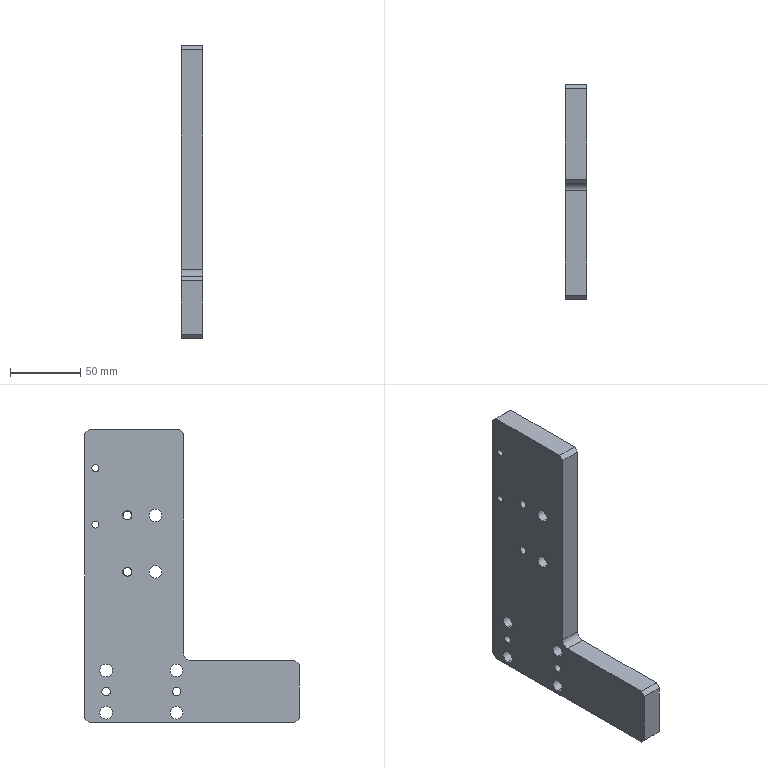Part | SolidWorks | features HoleWzd 9, Chamfer 1, Extrusion 1, Fillet 1, ICE 1 | 1 solid | 84 faces | box 15 x 152.1 x 208 mm | volume 261148 mm3 | cylinder 45 | cone 24 | plane 15 | commonest cylinder face diameters 5 x12 9 x12 4.2 x8 6 x8 15 x4 10 x1